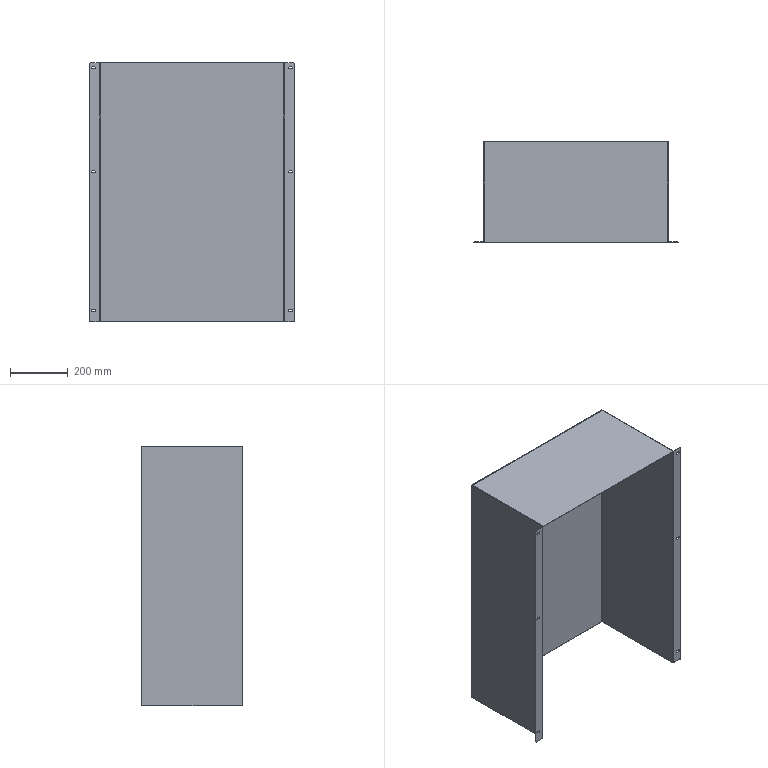Part | SolidWorks | features EdgeFlange 2, Fillet 1, FlatPattern 1, HoleWzd 1, ICE 1, SMBaseFlange 1, SheetMetal 1 | 1 solid | 74 faces | box 707.6 x 350 x 898 mm | volume 1775221 mm3 | plane 44 | cylinder 26 | spline 4 | commonest cylinder face diameters 7 x12 1.473 x5 3.873 x5 6 x4